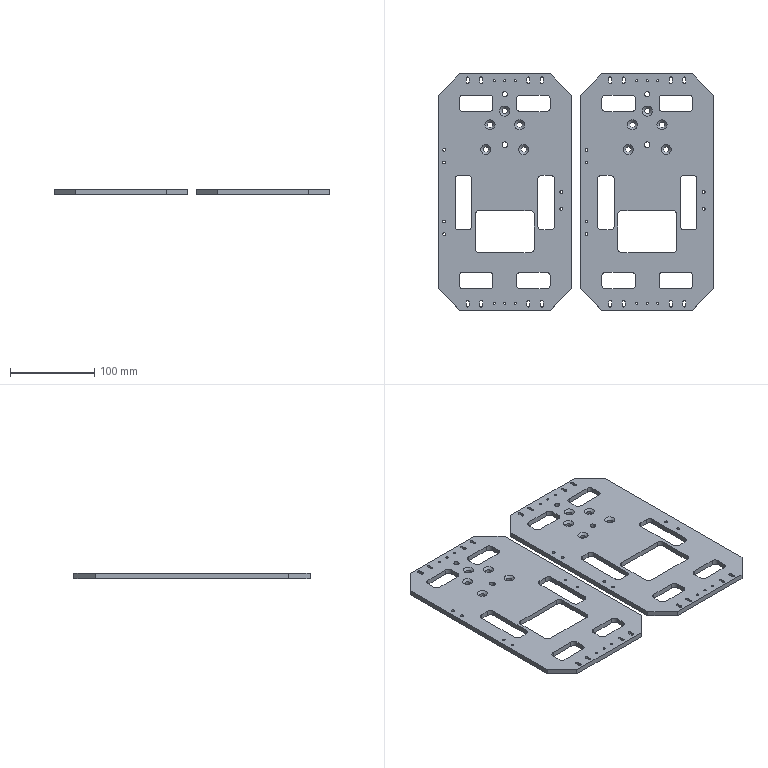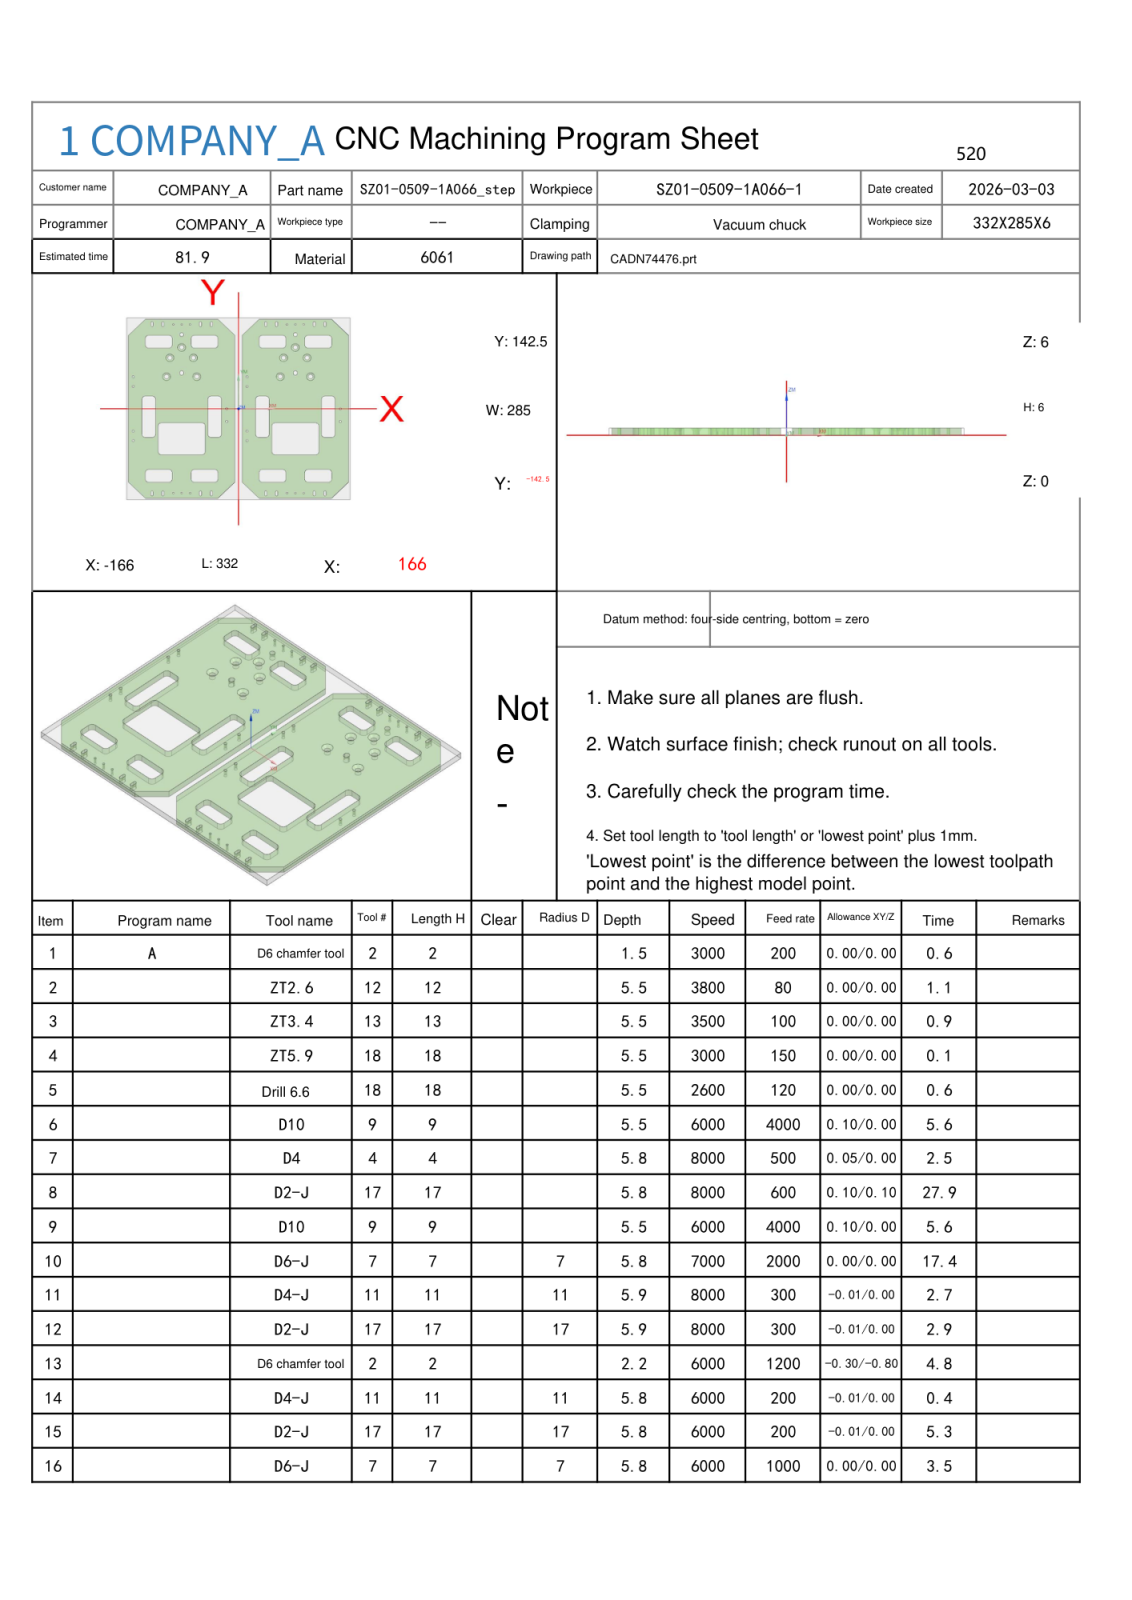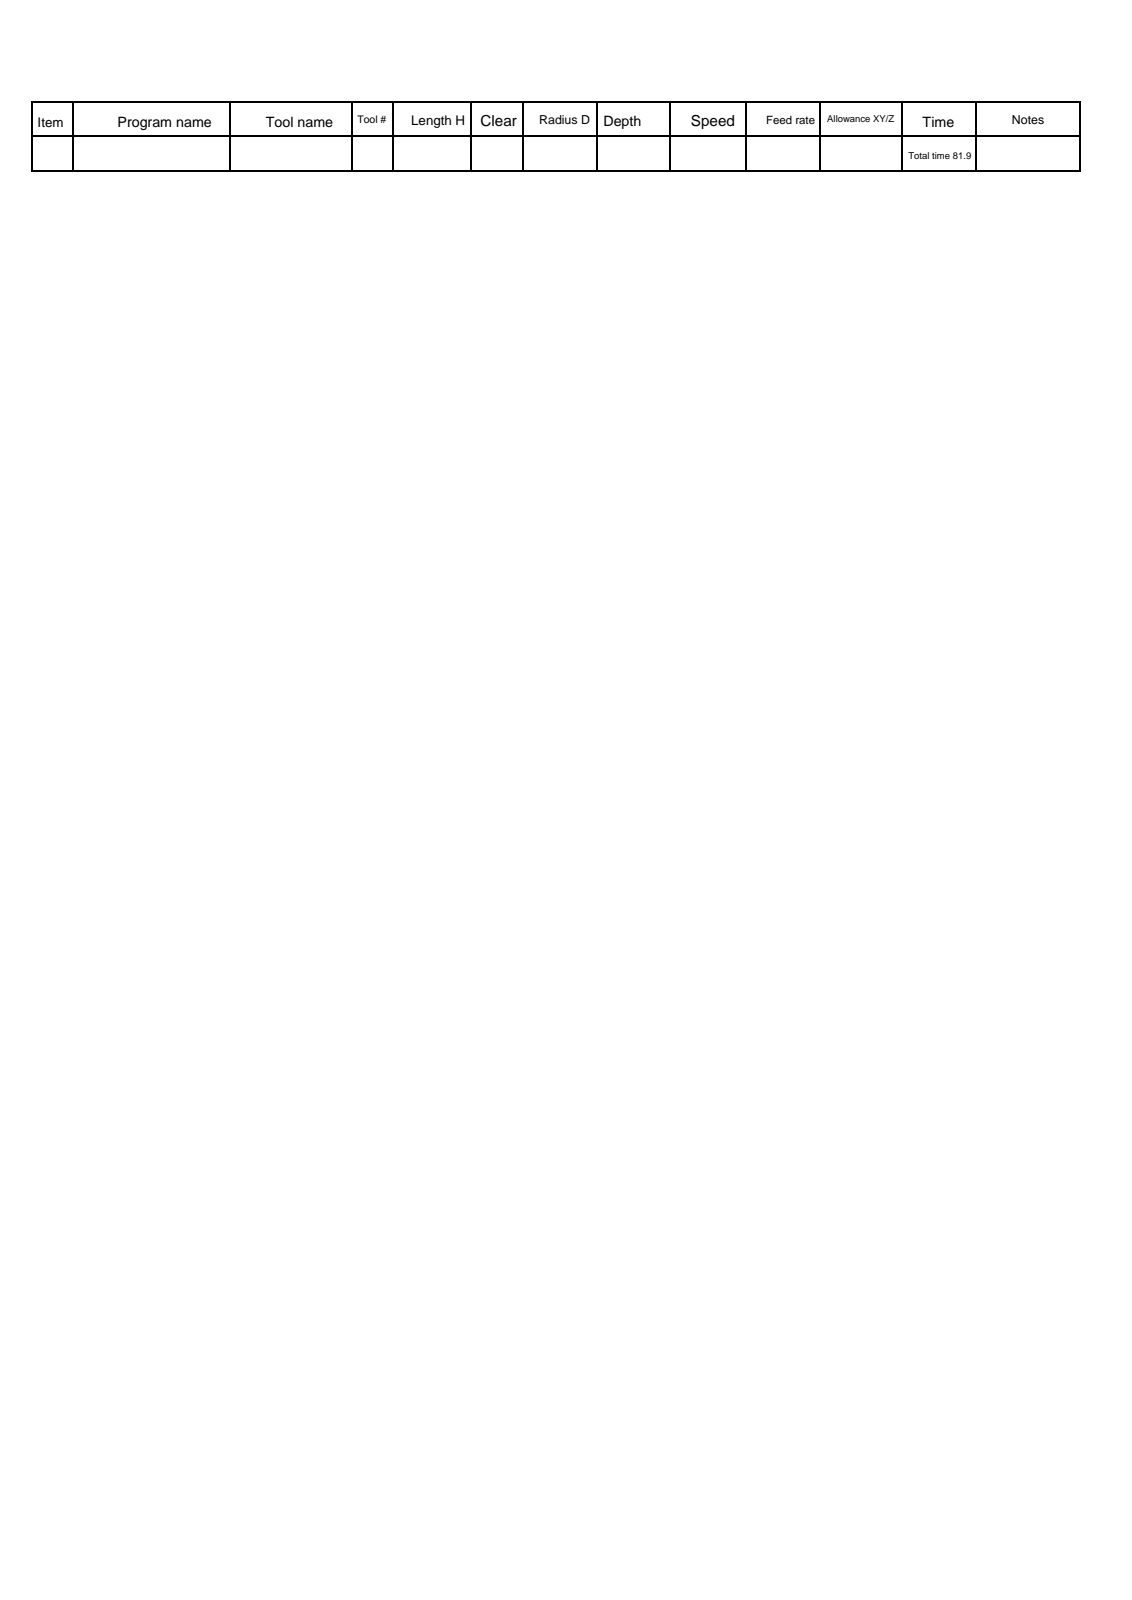NC program | NX | posted by the shop | part box 327 x 280 x 6 mm
Lines 1965 to 2845 of 31860:
N8 T17 M06
(D2-J  D=2. R=0. H=17 ce=0.10 di=0.10)
G00 G90 G54 X127.9 Y132.5 M03 S8000
G43 H17 Z36.
M08
Z6.5
G01 Y130.2 Z6.486 F600.
G03 X128.5 Y129.6 Z6.48 I.6 J0.0
X129.1 Y130.2 Z6.474 I0.0 J.6
G01 Y134.8 Z6.446
G03 X128.5 Y135.4 Z6.44 I-.6 J0.0
X127.9 Y134.8 Z6.434 I0.0 J-.6
G01 Y130.2 Z6.406
G03 X128.5 Y129.6 Z6.4 I.6 J0.0
X129.1 Y130.2 Z6.395 I0.0 J.6
G01 Y134.8 Z6.366
G03 X128.5 Y135.4 Z6.36 I-.6 J0.0
X127.9 Y134.8 Z6.355 I0.0 J-.6
G01 Y130.2 Z6.326
G03 X128.5 Y129.6 Z6.321 I.6 J0.0
X129.1 Y130.2 Z6.315 I0.0 J.6
G01 Y134.8 Z6.286
G03 X128.5 Y135.4 Z6.281 I-.6 J0.0
X127.9 Y134.8 Z6.275 I0.0 J-.6
G01 Y130.2 Z6.247
G03 X128.5 Y129.6 Z6.241 I.6 J0.0
X129.1 Y130.2 Z6.235 I0.0 J.6
G01 Y134.8 Z6.207
G03 X128.5 Y135.4 Z6.201 I-.6 J0.0
X127.9 Y134.8 Z6.195 I0.0 J-.6
G01 Y130.2 Z6.167
G03 X128.5 Y129.6 Z6.161 I.6 J0.0
X129.1 Y130.2 Z6.155 I0.0 J.6
G01 Y134.8 Z6.127
G03 X128.5 Y135.4 Z6.121 I-.6 J0.0
X127.9 Y134.8 Z6.115 I0.0 J-.6
G01 Y130.2 Z6.087
G03 X128.5 Y129.6 Z6.081 I.6 J0.0
X129.1 Y130.2 Z6.076 I0.0 J.6
G01 Y134.8 Z6.047
G03 X128.5 Y135.4 Z6.041 I-.6 J0.0
X127.9 Y134.8 Z6.036 I0.0 J-.6
G01 Y130.2 Z6.007
G03 X128.5 Y129.6 Z6.002 I.6 J0.0
X129.1 Y130.2 Z5.996 I0.0 J.6
G01 Y134.8 Z5.968
G03 X128.5 Y135.4 Z5.962 I-.6 J0.0
X127.9 Y134.8 Z5.956 I0.0 J-.6
G01 Y130.2 Z5.928
G03 X128.5 Y129.6 Z5.922 I.6 J0.0
X129.1 Y130.2 Z5.916 I0.0 J.6
G01 Y134.8 Z5.888
G03 X128.5 Y135.4 Z5.882 I-.6 J0.0
X127.9 Y134.8 Z5.876 I0.0 J-.6
G01 Y130.2 Z5.848
G03 X128.5 Y129.6 Z5.842 I.6 J0.0
X129.1 Y130.2 Z5.836 I0.0 J.6
G01 Y134.8 Z5.808
G03 X128.5 Y135.4 Z5.802 I-.6 J0.0
X127.9 Y134.8 Z5.796 I0.0 J-.6
G01 Y130.2 Z5.768
G03 X128.5 Y129.6 Z5.762 I.6 J0.0
X129.1 Y130.2 Z5.757 I0.0 J.6
G01 Y134.8 Z5.728
G03 X128.5 Y135.4 Z5.722 I-.6 J0.0
X127.9 Y134.8 Z5.717 I0.0 J-.6
G01 Y130.2 Z5.688
G03 X128.5 Y129.6 Z5.683 I.6 J0.0
X129.1 Y130.2 Z5.677 I0.0 J.6
G01 Y134.8 Z5.649
G03 X128.5 Y135.4 Z5.643 I-.6 J0.0
X127.9 Y134.8 Z5.637 I0.0 J-.6
G01 Y130.2 Z5.609
G03 X128.5 Y129.6 Z5.603 I.6 J0.0
X129.1 Y130.2 Z5.597 I0.0 J.6
G01 Y134.8 Z5.569
G03 X128.5 Y135.4 Z5.563 I-.6 J0.0
X127.9 Y134.8 Z5.557 I0.0 J-.6
G01 Y130.2 Z5.529
G03 X128.5 Y129.6 Z5.523 I.6 J0.0
X129.1 Y130.2 Z5.517 I0.0 J.6
G01 Y134.8 Z5.489
G03 X128.5 Y135.4 Z5.483 I-.6 J0.0
X127.9 Y134.8 Z5.477 I0.0 J-.6
G01 Y130.2 Z5.449
G03 X128.5 Y129.6 Z5.443 I.6 J0.0
X129.1 Y130.2 Z5.438 I0.0 J.6
G01 Y134.8 Z5.409
G03 X128.5 Y135.4 Z5.403 I-.6 J0.0
X127.9 Y134.8 Z5.398 I0.0 J-.6
G01 Y130.2 Z5.369
G03 X128.5 Y129.6 Z5.364 I.6 J0.0
X129.1 Y130.2 Z5.358 I0.0 J.6
G01 Y134.8 Z5.33
G03 X128.5 Y135.4 Z5.324 I-.6 J0.0
X127.9 Y134.8 Z5.318 I0.0 J-.6
G01 Y130.2 Z5.29
G03 X128.5 Y129.6 Z5.284 I.6 J0.0
X129.1 Y130.2 Z5.278 I0.0 J.6
G01 Y134.8 Z5.25
G03 X128.5 Y135.4 Z5.244 I-.6 J0.0
X127.9 Y134.8 Z5.238 I0.0 J-.6
G01 Y130.2 Z5.21
G03 X128.5 Y129.6 Z5.204 I.6 J0.0
X129.1 Y130.2 Z5.198 I0.0 J.6
G01 Y134.8 Z5.17
G03 X128.5 Y135.4 Z5.164 I-.6 J0.0
X127.9 Y134.8 Z5.158 I0.0 J-.6
G01 Y130.2 Z5.13
G03 X128.5 Y129.6 Z5.124 I.6 J0.0
X129.1 Y130.2 Z5.119 I0.0 J.6
G01 Y134.8 Z5.09
G03 X128.5 Y135.4 Z5.084 I-.6 J0.0
X127.9 Y134.8 Z5.079 I0.0 J-.6
G01 Y130.2 Z5.05
G03 X128.5 Y129.6 Z5.045 I.6 J0.0
X129.1 Y130.2 Z5.039 I0.0 J.6
G01 Y134.8 Z5.011
G03 X128.5 Y135.4 Z5.005 I-.6 J0.0
X127.9 Y134.8 Z4.999 I0.0 J-.6
G01 Y130.2 Z4.971
G03 X128.5 Y129.6 Z4.965 I.6 J0.0
X129.1 Y130.2 Z4.959 I0.0 J.6
G01 Y134.8 Z4.931
G03 X128.5 Y135.4 Z4.925 I-.6 J0.0
X127.9 Y134.8 Z4.919 I0.0 J-.6
G01 Y130.2 Z4.891
G03 X128.5 Y129.6 Z4.885 I.6 J0.0
X129.1 Y130.2 Z4.879 I0.0 J.6
G01 Y134.8 Z4.851
G03 X128.5 Y135.4 Z4.845 I-.6 J0.0
X127.9 Y134.8 Z4.839 I0.0 J-.6
G01 Y130.2 Z4.811
G03 X128.5 Y129.6 Z4.805 I.6 J0.0
X129.1 Y130.2 Z4.8 I0.0 J.6
G01 Y134.8 Z4.771
G03 X128.5 Y135.4 Z4.766 I-.6 J0.0
X127.9 Y134.8 Z4.76 I0.0 J-.6
G01 Y130.2 Z4.731
G03 X128.5 Y129.6 Z4.726 I.6 J0.0
X129.1 Y130.2 Z4.72 I0.0 J.6
G01 Y134.8 Z4.692
G03 X128.5 Y135.4 Z4.686 I-.6 J0.0
X127.9 Y134.8 Z4.68 I0.0 J-.6
G01 Y130.2 Z4.652
G03 X128.5 Y129.6 Z4.646 I.6 J0.0
X129.1 Y130.2 Z4.64 I0.0 J.6
G01 Y134.8 Z4.612
G03 X128.5 Y135.4 Z4.606 I-.6 J0.0
X127.9 Y134.8 Z4.6 I0.0 J-.6
G01 Y130.2 Z4.572
G03 X128.5 Y129.6 Z4.566 I.6 J0.0
X129.1 Y130.2 Z4.56 I0.0 J.6
G01 Y134.8 Z4.532
G03 X128.5 Y135.4 Z4.526 I-.6 J0.0
X127.9 Y134.8 Z4.52 I0.0 J-.6
G01 Y130.2 Z4.492
G03 X128.5 Y129.6 Z4.486 I.6 J0.0
X129.1 Y130.2 Z4.481 I0.0 J.6
G01 Y134.8 Z4.452
G03 X128.5 Y135.4 Z4.447 I-.6 J0.0
X127.9 Y134.8 Z4.441 I0.0 J-.6
G01 Y130.2 Z4.412
G03 X128.5 Y129.6 Z4.407 I.6 J0.0
X129.1 Y130.2 Z4.401 I0.0 J.6
G01 Y134.8 Z4.373
G03 X128.5 Y135.4 Z4.367 I-.6 J0.0
X127.9 Y134.8 Z4.361 I0.0 J-.6
G01 Y130.2 Z4.333
G03 X128.5 Y129.6 Z4.327 I.6 J0.0
X129.1 Y130.2 Z4.321 I0.0 J.6
G01 Y134.8 Z4.293
G03 X128.5 Y135.4 Z4.287 I-.6 J0.0
X127.9 Y134.8 Z4.281 I0.0 J-.6
G01 Y130.2 Z4.253
G03 X128.5 Y129.6 Z4.247 I.6 J0.0
X129.1 Y130.2 Z4.241 I0.0 J.6
G01 Y134.8 Z4.213
G03 X128.5 Y135.4 Z4.207 I-.6 J0.0
X127.9 Y134.8 Z4.201 I0.0 J-.6
G01 Y130.2 Z4.173
G03 X128.5 Y129.6 Z4.167 I.6 J0.0
X129.1 Y130.2 Z4.162 I0.0 J.6
G01 Y134.8 Z4.133
G03 X128.5 Y135.4 Z4.128 I-.6 J0.0
X127.9 Y134.8 Z4.122 I0.0 J-.6
G01 Y130.2 Z4.093
G03 X128.5 Y129.6 Z4.088 I.6 J0.0
X129.1 Y130.2 Z4.082 I0.0 J.6
G01 Y134.8 Z4.054
G03 X128.5 Y135.4 Z4.048 I-.6 J0.0
X127.9 Y134.8 Z4.042 I0.0 J-.6
G01 Y130.2 Z4.014
G03 X128.5 Y129.6 Z4.008 I.6 J0.0
X129.1 Y130.2 Z4.002 I0.0 J.6
G01 Y134.8 Z3.974
G03 X128.5 Y135.4 Z3.968 I-.6 J0.0
X127.9 Y134.8 Z3.962 I0.0 J-.6
G01 Y130.2 Z3.934
G03 X128.5 Y129.6 Z3.928 I.6 J0.0
X129.1 Y130.2 Z3.922 I0.0 J.6
G01 Y134.8 Z3.894
G03 X128.5 Y135.4 Z3.888 I-.6 J0.0
X127.9 Y134.8 Z3.882 I0.0 J-.6
G01 Y130.2 Z3.854
G03 X128.5 Y129.6 Z3.848 I.6 J0.0
X129.1 Y130.2 Z3.843 I0.0 J.6
G01 Y134.8 Z3.814
G03 X128.5 Y135.4 Z3.809 I-.6 J0.0
X127.9 Y134.8 Z3.803 I0.0 J-.6
G01 Y130.2 Z3.774
G03 X128.5 Y129.6 Z3.769 I.6 J0.0
X129.1 Y130.2 Z3.763 I0.0 J.6
G01 Y134.8 Z3.735
G03 X128.5 Y135.4 Z3.729 I-.6 J0.0
X127.9 Y134.8 Z3.723 I0.0 J-.6
G01 Y130.2 Z3.695
G03 X128.5 Y129.6 Z3.689 I.6 J0.0
X129.1 Y130.2 Z3.683 I0.0 J.6
G01 Y134.8 Z3.655
G03 X128.5 Y135.4 Z3.649 I-.6 J0.0
X127.9 Y134.8 Z3.643 I0.0 J-.6
G01 Y130.2 Z3.615
G03 X128.5 Y129.6 Z3.609 I.6 J0.0
X129.1 Y130.2 Z3.603 I0.0 J.6
G01 Y134.8 Z3.575
G03 X128.5 Y135.4 Z3.569 I-.6 J0.0
X127.9 Y134.8 Z3.564 I0.0 J-.6
G01 Y130.2 Z3.535
G03 X128.5 Y129.6 Z3.529 I.6 J0.0
X129.1 Y130.2 Z3.524 I0.0 J.6
G01 Y134.8 Z3.495
G03 X128.5 Y135.4 Z3.49 I-.6 J0.0
X127.9 Y134.8 Z3.484 I0.0 J-.6
G01 Y130.2 Z3.455
G03 X128.5 Y129.6 Z3.45 I.6 J0.0
X129.1 Y130.2 Z3.444 I0.0 J.6
G01 Y134.8 Z3.416
G03 X128.5 Y135.4 Z3.41 I-.6 J0.0
X127.9 Y134.8 Z3.404 I0.0 J-.6
G01 Y130.2 Z3.376
G03 X128.5 Y129.6 Z3.37 I.6 J0.0
X129.1 Y130.2 Z3.364 I0.0 J.6
G01 Y134.8 Z3.336
G03 X128.5 Y135.4 Z3.33 I-.6 J0.0
X127.9 Y134.8 Z3.324 I0.0 J-.6
G01 Y130.2 Z3.296
G03 X128.5 Y129.6 Z3.29 I.6 J0.0
X129.1 Y130.2 Z3.284 I0.0 J.6
G01 Y134.8 Z3.256
G03 X128.5 Y135.4 Z3.25 I-.6 J0.0
X127.9 Y134.8 Z3.245 I0.0 J-.6
G01 Y130.2 Z3.216
G03 X128.5 Y129.6 Z3.21 I.6 J0.0
X129.1 Y130.2 Z3.205 I0.0 J.6
G01 Y134.8 Z3.176
G03 X128.5 Y135.4 Z3.171 I-.6 J0.0
X127.9 Y134.8 Z3.165 I0.0 J-.6
G01 Y130.2 Z3.136
G03 X128.5 Y129.6 Z3.131 I.6 J0.0
X129.1 Y130.2 Z3.125 I0.0 J.6
G01 Y134.8 Z3.097
G03 X128.5 Y135.4 Z3.091 I-.6 J0.0
X127.9 Y134.8 Z3.085 I0.0 J-.6
G01 Y130.2 Z3.057
G03 X128.5 Y129.6 Z3.051 I.6 J0.0
X129.1 Y130.2 Z3.045 I0.0 J.6
G01 Y134.8 Z3.017
G03 X128.5 Y135.4 Z3.011 I-.6 J0.0
X127.9 Y134.8 Z3.005 I0.0 J-.6
G01 Y130.2 Z2.977
G03 X128.5 Y129.6 Z2.971 I.6 J0.0
X129.1 Y130.2 Z2.965 I0.0 J.6
G01 Y134.8 Z2.937
G03 X128.5 Y135.4 Z2.931 I-.6 J0.0
X127.9 Y134.8 Z2.926 I0.0 J-.6
G01 Y130.2 Z2.897
G03 X128.5 Y129.6 Z2.891 I.6 J0.0
X129.1 Y130.2 Z2.886 I0.0 J.6
G01 Y134.8 Z2.857
G03 X128.5 Y135.4 Z2.852 I-.6 J0.0
X127.9 Y134.8 Z2.846 I0.0 J-.6
G01 Y130.2 Z2.818
G03 X128.5 Y129.6 Z2.812 I.6 J0.0
X129.1 Y130.2 Z2.806 I0.0 J.6
G01 Y134.8 Z2.778
G03 X128.5 Y135.4 Z2.772 I-.6 J0.0
X127.9 Y134.8 Z2.766 I0.0 J-.6
G01 Y130.2 Z2.738
G03 X128.5 Y129.6 Z2.732 I.6 J0.0
X129.1 Y130.2 Z2.726 I0.0 J.6
G01 Y134.8 Z2.698
G03 X128.5 Y135.4 Z2.692 I-.6 J0.0
X127.9 Y134.8 Z2.686 I0.0 J-.6
G01 Y130.2 Z2.658
G03 X128.5 Y129.6 Z2.652 I.6 J0.0
X129.1 Y130.2 Z2.646 I0.0 J.6
G01 Y134.8 Z2.618
G03 X128.5 Y135.4 Z2.612 I-.6 J0.0
X127.9 Y134.8 Z2.607 I0.0 J-.6
G01 Y130.2 Z2.578
G03 X128.5 Y129.6 Z2.572 I.6 J0.0
X129.1 Y130.2 Z2.567 I0.0 J.6
G01 Y134.8 Z2.538
G03 X128.5 Y135.4 Z2.533 I-.6 J0.0
X127.9 Y134.8 Z2.527 I0.0 J-.6
G01 Y130.2 Z2.499
G03 X128.5 Y129.6 Z2.493 I.6 J0.0
X129.1 Y130.2 Z2.487 I0.0 J.6
G01 Y134.8 Z2.459
G03 X128.5 Y135.4 Z2.453 I-.6 J0.0
X127.9 Y134.8 Z2.447 I0.0 J-.6
G01 Y130.2 Z2.419
G03 X128.5 Y129.6 Z2.413 I.6 J0.0
X129.1 Y130.2 Z2.407 I0.0 J.6
G01 Y134.8 Z2.379
G03 X128.5 Y135.4 Z2.373 I-.6 J0.0
X127.9 Y134.8 Z2.367 I0.0 J-.6
G01 Y130.2 Z2.339
G03 X128.5 Y129.6 Z2.333 I.6 J0.0
X129.1 Y130.2 Z2.327 I0.0 J.6
G01 Y134.8 Z2.299
G03 X128.5 Y135.4 Z2.293 I-.6 J0.0
X127.9 Y134.8 Z2.288 I0.0 J-.6
G01 Y130.2 Z2.259
G03 X128.5 Y129.6 Z2.253 I.6 J0.0
X129.1 Y130.2 Z2.248 I0.0 J.6
G01 Y134.8 Z2.219
G03 X128.5 Y135.4 Z2.214 I-.6 J0.0
X127.9 Y134.8 Z2.208 I0.0 J-.6
G01 Y130.2 Z2.18
G03 X128.5 Y129.6 Z2.174 I.6 J0.0
X129.1 Y130.2 Z2.168 I0.0 J.6
G01 Y134.8 Z2.14
G03 X128.5 Y135.4 Z2.134 I-.6 J0.0
X127.9 Y134.8 Z2.128 I0.0 J-.6
G01 Y130.2 Z2.1
G03 X128.5 Y129.6 Z2.094 I.6 J0.0
X129.1 Y130.2 Z2.088 I0.0 J.6
G01 Y134.8 Z2.06
G03 X128.5 Y135.4 Z2.054 I-.6 J0.0
X127.9 Y134.8 Z2.048 I0.0 J-.6
G01 Y130.2 Z2.02
G03 X128.5 Y129.6 Z2.014 I.6 J0.0
X129.1 Y130.2 Z2.008 I0.0 J.6
G01 Y134.8 Z1.98
G03 X128.5 Y135.4 Z1.974 I-.6 J0.0
X127.9 Y134.8 Z1.969 I0.0 J-.6
G01 Y130.2 Z1.94
G03 X128.5 Y129.6 Z1.934 I.6 J0.0
X129.1 Y130.2 Z1.929 I0.0 J.6
G01 Y134.8 Z1.9
G03 X128.5 Y135.4 Z1.895 I-.6 J0.0
X127.9 Y134.8 Z1.889 I0.0 J-.6
G01 Y130.2 Z1.861
G03 X128.5 Y129.6 Z1.855 I.6 J0.0
X129.1 Y130.2 Z1.849 I0.0 J.6
G01 Y134.8 Z1.821
G03 X128.5 Y135.4 Z1.815 I-.6 J0.0
X127.9 Y134.8 Z1.809 I0.0 J-.6
G01 Y130.2 Z1.781
G03 X128.5 Y129.6 Z1.775 I.6 J0.0
X129.1 Y130.2 Z1.769 I0.0 J.6
G01 Y134.8 Z1.741
G03 X128.5 Y135.4 Z1.735 I-.6 J0.0
X127.9 Y134.8 Z1.729 I0.0 J-.6
G01 Y130.2 Z1.701
G03 X128.5 Y129.6 Z1.695 I.6 J0.0
X129.1 Y130.2 Z1.689 I0.0 J.6
G01 Y134.8 Z1.661
G03 X128.5 Y135.4 Z1.655 I-.6 J0.0
X127.9 Y134.8 Z1.65 I0.0 J-.6
G01 Y130.2 Z1.621
G03 X128.5 Y129.6 Z1.616 I.6 J0.0
X129.1 Y130.2 Z1.61 I0.0 J.6
G01 Y134.8 Z1.581
G03 X128.5 Y135.4 Z1.576 I-.6 J0.0
X127.9 Y134.8 Z1.57 I0.0 J-.6
G01 Y130.2 Z1.542
G03 X128.5 Y129.6 Z1.536 I.6 J0.0
X129.1 Y130.2 Z1.53 I0.0 J.6
G01 Y134.8 Z1.502
G03 X128.5 Y135.4 Z1.496 I-.6 J0.0
X127.9 Y134.8 Z1.49 I0.0 J-.6
G01 Y130.2 Z1.462
G03 X128.5 Y129.6 Z1.456 I.6 J0.0
X129.1 Y130.2 Z1.45 I0.0 J.6
G01 Y134.8 Z1.422
G03 X128.5 Y135.4 Z1.416 I-.6 J0.0
X127.9 Y134.8 Z1.41 I0.0 J-.6
G01 Y130.2 Z1.382
G03 X128.5 Y129.6 Z1.376 I.6 J0.0
X129.1 Y130.2 Z1.37 I0.0 J.6
G01 Y134.8 Z1.342
G03 X128.5 Y135.4 Z1.336 I-.6 J0.0
X127.9 Y134.8 Z1.331 I0.0 J-.6
G01 Y130.2 Z1.302
G03 X128.5 Y129.6 Z1.297 I.6 J0.0
X129.1 Y130.2 Z1.291 I0.0 J.6
G01 Y134.8 Z1.262
G03 X128.5 Y135.4 Z1.257 I-.6 J0.0
X127.9 Y134.8 Z1.251 I0.0 J-.6
G01 Y130.2 Z1.223
G03 X128.5 Y129.6 Z1.217 I.6 J0.0
X129.1 Y130.2 Z1.211 I0.0 J.6
G01 Y134.8 Z1.183
G03 X128.5 Y135.4 Z1.177 I-.6 J0.0
X127.9 Y134.8 Z1.171 I0.0 J-.6
G01 Y130.2 Z1.143
G03 X128.5 Y129.6 Z1.137 I.6 J0.0
X129.1 Y130.2 Z1.131 I0.0 J.6
G01 Y134.8 Z1.103
G03 X128.5 Y135.4 Z1.097 I-.6 J0.0
X127.9 Y134.8 Z1.091 I0.0 J-.6
G01 Y130.2 Z1.063
G03 X128.5 Y129.6 Z1.057 I.6 J0.0
X129.1 Y130.2 Z1.051 I0.0 J.6
G01 Y134.8 Z1.023
G03 X128.5 Y135.4 Z1.017 I-.6 J0.0
X127.9 Y134.8 Z1.012 I0.0 J-.6
G01 Y130.2 Z.983
G03 X128.5 Y129.6 Z.978 I.6 J0.0
X129.1 Y130.2 Z.972 I0.0 J.6
G01 Y134.8 Z.943
G03 X128.5 Y135.4 Z.938 I-.6 J0.0
X127.9 Y134.8 Z.932 I0.0 J-.6
G01 Y130.2 Z.904
G03 X128.5 Y129.6 Z.898 I.6 J0.0
X129.1 Y130.2 Z.892 I0.0 J.6
G01 Y134.8 Z.864
G03 X128.5 Y135.4 Z.858 I-.6 J0.0
X127.9 Y134.8 Z.852 I0.0 J-.6
G01 Y130.2 Z.824
G03 X128.5 Y129.6 Z.818 I.6 J0.0
X129.1 Y130.2 Z.812 I0.0 J.6
G01 Y134.8 Z.784
G03 X128.5 Y135.4 Z.778 I-.6 J0.0
X127.9 Y134.8 Z.772 I0.0 J-.6
G01 Y130.2 Z.744
G03 X128.5 Y129.6 Z.738 I.6 J0.0
X129.1 Y130.2 Z.732 I0.0 J.6
G01 Y134.8 Z.704
G03 X128.5 Y135.4 Z.698 I-.6 J0.0
X127.9 Y134.8 Z.693 I0.0 J-.6
G01 Y130.2 Z.664
G03 X128.5 Y129.6 Z.659 I.6 J0.0
X129.1 Y130.2 Z.653 I0.0 J.6
G01 Y134.8 Z.624
G03 X128.5 Y135.4 Z.619 I-.6 J0.0
X127.9 Y134.8 Z.613 I0.0 J-.6
G01 Y130.2 Z.585
G03 X128.5 Y129.6 Z.579 I.6 J0.0
X129.1 Y130.2 Z.573 I0.0 J.6
G01 Y134.8 Z.545
G03 X128.5 Y135.4 Z.539 I-.6 J0.0
X127.9 Y134.8 Z.533 I0.0 J-.6
G01 Y130.2 Z.505
G03 X128.5 Y129.6 Z.499 I.6 J0.0
X129.1 Y130.2 Z.493 I0.0 J.6
G01 Y134.8 Z.465
G03 X128.5 Y135.4 Z.459 I-.6 J0.0
X127.9 Y134.8 Z.453 I0.0 J-.6
G01 Y130.2 Z.425
G03 X128.5 Y129.6 Z.419 I.6 J0.0
X129.1 Y130.2 Z.414 I0.0 J.6
G01 Y134.8 Z.385
G03 X128.5 Y135.4 Z.379 I-.6 J0.0
X127.9 Y134.8 Z.374 I0.0 J-.6
G01 Y130.2 Z.345
G03 X128.5 Y129.6 Z.34 I.6 J0.0
X129.1 Y130.2 Z.334 I0.0 J.6
G01 Y134.8 Z.305
G03 X128.5 Y135.4 Z.3 I-.6 J0.0
X127.9 Y134.8 Z.294 I0.0 J-.6
G01 Y130.2 Z.266
G03 X128.5 Y129.6 Z.26 I.6 J0.0
X129.1 Y130.2 Z.254 I0.0 J.6
G01 Y134.8 Z.226
G03 X128.5 Y135.4 Z.22 I-.6 J0.0
X127.9 Y134.8 Z.214 I0.0 J-.6
G01 Y132.5 Z.2
Y130.2
G03 X128.5 Y129.6 I.6 J0.0
X129.1 Y130.2 I0.0 J.6
G01 Y134.8
G03 X128.5 Y135.4 I-.6 J0.0
X127.9 Y134.8 I0.0 J-.6
G01 Y132.5
Y132.
Z1.2
G00 Z36.
X113.1 Y132.5
Z6.5
G01 Y134.8 Z6.486
G03 X112.5 Y135.4 Z6.48 I-.6 J0.0
X111.9 Y134.8 Z6.474 I0.0 J-.6
G01 Y130.2 Z6.446
G03 X112.5 Y129.6 Z6.44 I.6 J0.0
X113.1 Y130.2 Z6.434 I0.0 J.6
G01 Y134.8 Z6.406
G03 X112.5 Y135.4 Z6.4 I-.6 J0.0
X111.9 Y134.8 Z6.395 I0.0 J-.6
G01 Y130.2 Z6.366
G03 X112.5 Y129.6 Z6.36 I.6 J0.0
X113.1 Y130.2 Z6.355 I0.0 J.6
G01 Y134.8 Z6.326
G03 X112.5 Y135.4 Z6.321 I-.6 J0.0
X111.9 Y134.8 Z6.315 I0.0 J-.6
G01 Y130.2 Z6.286
G03 X112.5 Y129.6 Z6.281 I.6 J0.0
X113.1 Y130.2 Z6.275 I0.0 J.6
G01 Y134.8 Z6.247
G03 X112.5 Y135.4 Z6.241 I-.6 J0.0
X111.9 Y134.8 Z6.235 I0.0 J-.6
G01 Y130.2 Z6.207
G03 X112.5 Y129.6 Z6.201 I.6 J0.0
X113.1 Y130.2 Z6.195 I0.0 J.6
G01 Y134.8 Z6.167
G03 X112.5 Y135.4 Z6.161 I-.6 J0.0
X111.9 Y134.8 Z6.155 I0.0 J-.6
G01 Y130.2 Z6.127
G03 X112.5 Y129.6 Z6.121 I.6 J0.0
X113.1 Y130.2 Z6.115 I0.0 J.6
G01 Y134.8 Z6.087
G03 X112.5 Y135.4 Z6.081 I-.6 J0.0
X111.9 Y134.8 Z6.076 I0.0 J-.6
G01 Y130.2 Z6.047
G03 X112.5 Y129.6 Z6.041 I.6 J0.0
X113.1 Y130.2 Z6.036 I0.0 J.6
G01 Y134.8 Z6.007
G03 X112.5 Y135.4 Z6.002 I-.6 J0.0
X111.9 Y134.8 Z5.996 I0.0 J-.6
G01 Y130.2 Z5.968
G03 X112.5 Y129.6 Z5.962 I.6 J0.0
X113.1 Y130.2 Z5.956 I0.0 J.6
G01 Y134.8 Z5.928
G03 X112.5 Y135.4 Z5.922 I-.6 J0.0
X111.9 Y134.8 Z5.916 I0.0 J-.6
G01 Y130.2 Z5.888
G03 X112.5 Y129.6 Z5.882 I.6 J0.0
X113.1 Y130.2 Z5.876 I0.0 J.6
G01 Y134.8 Z5.848
G03 X112.5 Y135.4 Z5.842 I-.6 J0.0
X111.9 Y134.8 Z5.836 I0.0 J-.6
G01 Y130.2 Z5.808
G03 X112.5 Y129.6 Z5.802 I.6 J0.0
X113.1 Y130.2 Z5.796 I0.0 J.6
G01 Y134.8 Z5.768
G03 X112.5 Y135.4 Z5.762 I-.6 J0.0
X111.9 Y134.8 Z5.757 I0.0 J-.6
G01 Y130.2 Z5.728
G03 X112.5 Y129.6 Z5.722 I.6 J0.0
X113.1 Y130.2 Z5.717 I0.0 J.6
G01 Y134.8 Z5.688
G03 X112.5 Y135.4 Z5.683 I-.6 J0.0
X111.9 Y134.8 Z5.677 I0.0 J-.6
G01 Y130.2 Z5.649
G03 X112.5 Y129.6 Z5.643 I.6 J0.0
X113.1 Y130.2 Z5.637 I0.0 J.6
G01 Y134.8 Z5.609
G03 X112.5 Y135.4 Z5.603 I-.6 J0.0
X111.9 Y134.8 Z5.597 I0.0 J-.6
G01 Y130.2 Z5.569
G03 X112.5 Y129.6 Z5.563 I.6 J0.0
X113.1 Y130.2 Z5.557 I0.0 J.6
G01 Y134.8 Z5.529
G03 X112.5 Y135.4 Z5.523 I-.6 J0.0
X111.9 Y134.8 Z5.517 I0.0 J-.6
G01 Y130.2 Z5.489
G03 X112.5 Y129.6 Z5.483 I.6 J0.0
X113.1 Y130.2 Z5.477 I0.0 J.6
G01 Y134.8 Z5.449
G03 X112.5 Y135.4 Z5.443 I-.6 J0.0
X111.9 Y134.8 Z5.438 I0.0 J-.6
G01 Y130.2 Z5.409
G03 X112.5 Y129.6 Z5.403 I.6 J0.0
X113.1 Y130.2 Z5.398 I0.0 J.6
G01 Y134.8 Z5.369
G03 X112.5 Y135.4 Z5.364 I-.6 J0.0
X111.9 Y134.8 Z5.358 I0.0 J-.6
G01 Y130.2 Z5.33
G03 X112.5 Y129.6 Z5.324 I.6 J0.0
X113.1 Y130.2 Z5.318 I0.0 J.6
G01 Y134.8 Z5.29
G03 X112.5 Y135.4 Z5.284 I-.6 J0.0
X111.9 Y134.8 Z5.278 I0.0 J-.6
G01 Y130.2 Z5.25
G03 X112.5 Y129.6 Z5.244 I.6 J0.0
X113.1 Y130.2 Z5.238 I0.0 J.6
G01 Y134.8 Z5.21
G03 X112.5 Y135.4 Z5.204 I-.6 J0.0
X111.9 Y134.8 Z5.198 I0.0 J-.6
G01 Y130.2 Z5.17
G03 X112.5 Y129.6 Z5.164 I.6 J0.0
X113.1 Y130.2 Z5.158 I0.0 J.6
G01 Y134.8 Z5.13
G03 X112.5 Y135.4 Z5.124 I-.6 J0.0
X111.9 Y134.8 Z5.119 I0.0 J-.6
G01 Y130.2 Z5.09
G03 X112.5 Y129.6 Z5.084 I.6 J0.0
X113.1 Y130.2 Z5.079 I0.0 J.6
G01 Y134.8 Z5.05
G03 X112.5 Y135.4 Z5.045 I-.6 J0.0
X111.9 Y134.8 Z5.039 I0.0 J-.6
G01 Y130.2 Z5.011
G03 X112.5 Y129.6 Z5.005 I.6 J0.0
X113.1 Y130.2 Z4.999 I0.0 J.6
G01 Y134.8 Z4.971
G03 X112.5 Y135.4 Z4.965 I-.6 J0.0
X111.9 Y134.8 Z4.959 I0.0 J-.6
G01 Y130.2 Z4.931
G03 X112.5 Y129.6 Z4.925 I.6 J0.0
X113.1 Y130.2 Z4.919 I0.0 J.6
G01 Y134.8 Z4.891
G03 X112.5 Y135.4 Z4.885 I-.6 J0.0
X111.9 Y134.8 Z4.879 I0.0 J-.6
G01 Y130.2 Z4.851
G03 X112.5 Y129.6 Z4.845 I.6 J0.0
X113.1 Y130.2 Z4.839 I0.0 J.6
G01 Y134.8 Z4.811
G03 X112.5 Y135.4 Z4.805 I-.6 J0.0
X111.9 Y134.8 Z4.8 I0.0 J-.6
G01 Y130.2 Z4.771
G03 X112.5 Y129.6 Z4.766 I.6 J0.0
X113.1 Y130.2 Z4.76 I0.0 J.6
G01 Y134.8 Z4.731
G03 X112.5 Y135.4 Z4.726 I-.6 J0.0
X111.9 Y134.8 Z4.72 I0.0 J-.6
G01 Y130.2 Z4.692
G03 X112.5 Y129.6 Z4.686 I.6 J0.0
X113.1 Y130.2 Z4.68 I0.0 J.6
G01 Y134.8 Z4.652
G03 X112.5 Y135.4 Z4.646 I-.6 J0.0
X111.9 Y134.8 Z4.64 I0.0 J-.6
G01 Y130.2 Z4.612
G03 X112.5 Y129.6 Z4.606 I.6 J0.0
X113.1 Y130.2 Z4.6 I0.0 J.6
G01 Y134.8 Z4.572
G03 X112.5 Y135.4 Z4.566 I-.6 J0.0
X111.9 Y134.8 Z4.56 I0.0 J-.6
G01 Y130.2 Z4.532
G03 X112.5 Y129.6 Z4.526 I.6 J0.0
X113.1 Y130.2 Z4.52 I0.0 J.6
G01 Y134.8 Z4.492
G03 X112.5 Y135.4 Z4.486 I-.6 J0.0
X111.9 Y134.8 Z4.481 I0.0 J-.6
G01 Y130.2 Z4.452
G03 X112.5 Y129.6 Z4.447 I.6 J0.0
X113.1 Y130.2 Z4.441 I0.0 J.6
G01 Y134.8 Z4.412
G03 X112.5 Y135.4 Z4.407 I-.6 J0.0
X111.9 Y134.8 Z4.401 I0.0 J-.6
G01 Y130.2 Z4.373
G03 X112.5 Y129.6 Z4.367 I.6 J0.0
X113.1 Y130.2 Z4.361 I0.0 J.6
G01 Y134.8 Z4.333
G03 X112.5 Y135.4 Z4.327 I-.6 J0.0
X111.9 Y134.8 Z4.321 I0.0 J-.6
G01 Y130.2 Z4.293
G03 X112.5 Y129.6 Z4.287 I.6 J0.0
X113.1 Y130.2 Z4.281 I0.0 J.6
G01 Y134.8 Z4.253
G03 X112.5 Y135.4 Z4.247 I-.6 J0.0
X111.9 Y134.8 Z4.241 I0.0 J-.6
G01 Y130.2 Z4.213
G03 X112.5 Y129.6 Z4.207 I.6 J0.0
X113.1 Y130.2 Z4.201 I0.0 J.6
G01 Y134.8 Z4.173
G03 X112.5 Y135.4 Z4.167 I-.6 J0.0
X111.9 Y134.8 Z4.162 I0.0 J-.6
G01 Y130.2 Z4.133
G03 X112.5 Y129.6 Z4.128 I.6 J0.0
X113.1 Y130.2 Z4.122 I0.0 J.6
G01 Y134.8 Z4.093
G03 X112.5 Y135.4 Z4.088 I-.6 J0.0
X111.9 Y134.8 Z4.082 I0.0 J-.6
G01 Y130.2 Z4.054
G03 X112.5 Y129.6 Z4.048 I.6 J0.0
X113.1 Y130.2 Z4.042 I0.0 J.6
G01 Y134.8 Z4.014
G03 X112.5 Y135.4 Z4.008 I-.6 J0.0
X111.9 Y134.8 Z4.002 I0.0 J-.6
G01 Y130.2 Z3.974
G03 X112.5 Y129.6 Z3.968 I.6 J0.0
X113.1 Y130.2 Z3.962 I0.0 J.6
G01 Y134.8 Z3.934
G03 X112.5 Y135.4 Z3.928 I-.6 J0.0
X111.9 Y134.8 Z3.922 I0.0 J-.6
G01 Y130.2 Z3.894
G03 X112.5 Y129.6 Z3.888 I.6 J0.0
X113.1 Y130.2 Z3.882 I0.0 J.6
G01 Y134.8 Z3.854
G03 X112.5 Y135.4 Z3.848 I-.6 J0.0
X111.9 Y134.8 Z3.843 I0.0 J-.6
G01 Y130.2 Z3.814
G03 X112.5 Y129.6 Z3.809 I.6 J0.0
X113.1 Y130.2 Z3.803 I0.0 J.6
G01 Y134.8 Z3.774
G03 X112.5 Y135.4 Z3.769 I-.6 J0.0
X111.9 Y134.8 Z3.763 I0.0 J-.6
G01 Y130.2 Z3.735
G03 X112.5 Y129.6 Z3.729 I.6 J0.0
X113.1 Y130.2 Z3.723 I0.0 J.6
G01 Y134.8 Z3.695
G03 X112.5 Y135.4 Z3.689 I-.6 J0.0
X111.9 Y134.8 Z3.683 I0.0 J-.6
G01 Y130.2 Z3.655
G03 X112.5 Y129.6 Z3.649 I.6 J0.0
X113.1 Y130.2 Z3.643 I0.0 J.6
G01 Y134.8 Z3.615
G03 X112.5 Y135.4 Z3.609 I-.6 J0.0
X111.9 Y134.8 Z3.603 I0.0 J-.6
G01 Y130.2 Z3.575
G03 X112.5 Y129.6 Z3.569 I.6 J0.0
X113.1 Y130.2 Z3.564 I0.0 J.6
G01 Y134.8 Z3.535
G03 X112.5 Y135.4 Z3.529 I-.6 J0.0
X111.9 Y134.8 Z3.524 I0.0 J-.6
G01 Y130.2 Z3.495
G03 X112.5 Y129.6 Z3.49 I.6 J0.0
X113.1 Y130.2 Z3.484 I0.0 J.6
G01 Y134.8 Z3.455
G03 X112.5 Y135.4 Z3.45 I-.6 J0.0
X111.9 Y134.8 Z3.444 I0.0 J-.6
G01 Y130.2 Z3.416
G03 X112.5 Y129.6 Z3.41 I.6 J0.0
X113.1 Y130.2 Z3.404 I0.0 J.6
G01 Y134.8 Z3.376
G03 X112.5 Y135.4 Z3.37 I-.6 J0.0
X111.9 Y134.8 Z3.364 I0.0 J-.6
G01 Y130.2 Z3.336
G03 X112.5 Y129.6 Z3.33 I.6 J0.0
X113.1 Y130.2 Z3.324 I0.0 J.6
G01 Y134.8 Z3.296
G03 X112.5 Y135.4 Z3.29 I-.6 J0.0
X111.9 Y134.8 Z3.284 I0.0 J-.6
G01 Y130.2 Z3.256
G03 X112.5 Y129.6 Z3.25 I.6 J0.0
X113.1 Y130.2 Z3.245 I0.0 J.6
G01 Y134.8 Z3.216
G03 X112.5 Y135.4 Z3.21 I-.6 J0.0
X111.9 Y134.8 Z3.205 I0.0 J-.6
G01 Y130.2 Z3.176
G03 X112.5 Y129.6 Z3.171 I.6 J0.0
X113.1 Y130.2 Z3.165 I0.0 J.6
G01 Y134.8 Z3.136
G03 X112.5 Y135.4 Z3.131 I-.6 J0.0
X111.9 Y134.8 Z3.125 I0.0 J-.6
G01 Y130.2 Z3.097
G03 X112.5 Y129.6 Z3.091 I.6 J0.0
X113.1 Y130.2 Z3.085 I0.0 J.6
G01 Y134.8 Z3.057
G03 X112.5 Y135.4 Z3.051 I-.6 J0.0
X111.9 Y134.8 Z3.045 I0.0 J-.6
G01 Y130.2 Z3.017
G03 X112.5 Y129.6 Z3.011 I.6 J0.0
X113.1 Y130.2 Z3.005 I0.0 J.6
G01 Y134.8 Z2.977
G03 X112.5 Y135.4 Z2.971 I-.6 J0.0
X111.9 Y134.8 Z2.965 I0.0 J-.6
G01 Y130.2 Z2.937
G03 X112.5 Y129.6 Z2.931 I.6 J0.0
X113.1 Y130.2 Z2.926 I0.0 J.6
G01 Y134.8 Z2.897
G03 X112.5 Y135.4 Z2.891 I-.6 J0.0
X111.9 Y134.8 Z2.886 I0.0 J-.6
G01 Y130.2 Z2.857
G03 X112.5 Y129.6 Z2.852 I.6 J0.0
X113.1 Y130.2 Z2.846 I0.0 J.6
G01 Y134.8 Z2.818
G03 X112.5 Y135.4 Z2.812 I-.6 J0.0
X111.9 Y134.8 Z2.806 I0.0 J-.6
G01 Y130.2 Z2.778
G03 X112.5 Y129.6 Z2.772 I.6 J0.0
X113.1 Y130.2 Z2.766 I0.0 J.6
G01 Y134.8 Z2.738
G03 X112.5 Y135.4 Z2.732 I-.6 J0.0
X111.9 Y134.8 Z2.726 I0.0 J-.6
G01 Y130.2 Z2.698
G03 X112.5 Y129.6 Z2.692 I.6 J0.0
X113.1 Y130.2 Z2.686 I0.0 J.6
G01 Y134.8 Z2.658
G03 X112.5 Y135.4 Z2.652 I-.6 J0.0
X111.9 Y134.8 Z2.646 I0.0 J-.6
G01 Y130.2 Z2.618
G03 X112.5 Y129.6 Z2.612 I.6 J0.0
X113.1 Y130.2 Z2.607 I0.0 J.6
G01 Y134.8 Z2.578
G03 X112.5 Y135.4 Z2.572 I-.6 J0.0
X111.9 Y134.8 Z2.567 I0.0 J-.6
G01 Y130.2 Z2.538
G03 X112.5 Y129.6 Z2.533 I.6 J0.0
X113.1 Y130.2 Z2.527 I0.0 J.6
G01 Y134.8 Z2.499
G03 X112.5 Y135.4 Z2.493 I-.6 J0.0
X111.9 Y134.8 Z2.487 I0.0 J-.6
G01 Y130.2 Z2.459
G03 X112.5 Y129.6 Z2.453 I.6 J0.0
X113.1 Y130.2 Z2.447 I0.0 J.6
G01 Y134.8 Z2.419
G03 X112.5 Y135.4 Z2.413 I-.6 J0.0
X111.9 Y134.8 Z2.407 I0.0 J-.6
G01 Y130.2 Z2.379
G03 X112.5 Y129.6 Z2.373 I.6 J0.0
X113.1 Y130.2 Z2.367 I0.0 J.6
G01 Y134.8 Z2.339
G03 X112.5 Y135.4 Z2.333 I-.6 J0.0
X111.9 Y134.8 Z2.327 I0.0 J-.6
G01 Y130.2 Z2.299
G03 X112.5 Y129.6 Z2.293 I.6 J0.0
X113.1 Y130.2 Z2.288 I0.0 J.6
G01 Y134.8 Z2.259
G03 X112.5 Y135.4 Z2.253 I-.6 J0.0
X111.9 Y134.8 Z2.248 I0.0 J-.6
G01 Y130.2 Z2.219
G03 X112.5 Y129.6 Z2.214 I.6 J0.0
X113.1 Y130.2 Z2.208 I0.0 J.6
G01 Y134.8 Z2.18
G03 X112.5 Y135.4 Z2.174 I-.6 J0.0
X111.9 Y134.8 Z2.168 I0.0 J-.6
G01 Y130.2 Z2.14
G03 X112.5 Y129.6 Z2.134 I.6 J0.0
X113.1 Y130.2 Z2.128 I0.0 J.6
G01 Y134.8 Z2.1
G03 X112.5 Y135.4 Z2.094 I-.6 J0.0
X111.9 Y134.8 Z2.088 I0.0 J-.6
G01 Y130.2 Z2.06
G03 X112.5 Y129.6 Z2.054 I.6 J0.0
X113.1 Y130.2 Z2.048 I0.0 J.6
G01 Y134.8 Z2.02
G03 X112.5 Y135.4 Z2.014 I-.6 J0.0
X111.9 Y134.8 Z2.008 I0.0 J-.6
G01 Y130.2 Z1.98
G03 X112.5 Y129.6 Z1.974 I.6 J0.0
X113.1 Y130.2 Z1.969 I0.0 J.6
G01 Y134.8 Z1.94
G03 X112.5 Y135.4 Z1.934 I-.6 J0.0
X111.9 Y134.8 Z1.929 I0.0 J-.6
G01 Y130.2 Z1.9
G03 X112.5 Y129.6 Z1.895 I.6 J0.0
X113.1 Y130.2 Z1.889 I0.0 J.6
G01 Y134.8 Z1.861
G03 X112.5 Y135.4 Z1.855 I-.6 J0.0
X111.9 Y134.8 Z1.849 I0.0 J-.6
G01 Y130.2 Z1.821
G03 X112.5 Y129.6 Z1.815 I.6 J0.0
X113.1 Y130.2 Z1.809 I0.0 J.6
G01 Y134.8 Z1.781
G03 X112.5 Y135.4 Z1.775 I-.6 J0.0
X111.9 Y134.8 Z1.769 I0.0 J-.6
G01 Y130.2 Z1.741
G03 X112.5 Y129.6 Z1.735 I.6 J0.0
X113.1 Y130.2 Z1.729 I0.0 J.6
G01 Y134.8 Z1.701
G03 X112.5 Y135.4 Z1.695 I-.6 J0.0
X111.9 Y134.8 Z1.689 I0.0 J-.6
G01 Y130.2 Z1.661
G03 X112.5 Y129.6 Z1.655 I.6 J0.0
X113.1 Y130.2 Z1.65 I0.0 J.6
G01 Y134.8 Z1.621
G03 X112.5 Y135.4 Z1.616 I-.6 J0.0
X111.9 Y134.8 Z1.61 I0.0 J-.6
G01 Y130.2 Z1.581
G03 X112.5 Y129.6 Z1.576 I.6 J0.0
X113.1 Y130.2 Z1.57 I0.0 J.6
G01 Y134.8 Z1.542
G03 X112.5 Y135.4 Z1.536 I-.6 J0.0
X111.9 Y134.8 Z1.53 I0.0 J-.6
G01 Y130.2 Z1.502
G03 X112.5 Y129.6 Z1.496 I.6 J0.0
X113.1 Y130.2 Z1.49 I0.0 J.6
G01 Y134.8 Z1.462
G03 X112.5 Y135.4 Z1.456 I-.6 J0.0
X111.9 Y134.8 Z1.45 I0.0 J-.6
G01 Y130.2 Z1.422
G03 X112.5 Y129.6 Z1.416 I.6 J0.0
X113.1 Y130.2 Z1.41 I0.0 J.6
G01 Y134.8 Z1.382
G03 X112.5 Y135.4 Z1.376 I-.6 J0.0
X111.9 Y134.8 Z1.37 I0.0 J-.6
G01 Y130.2 Z1.342